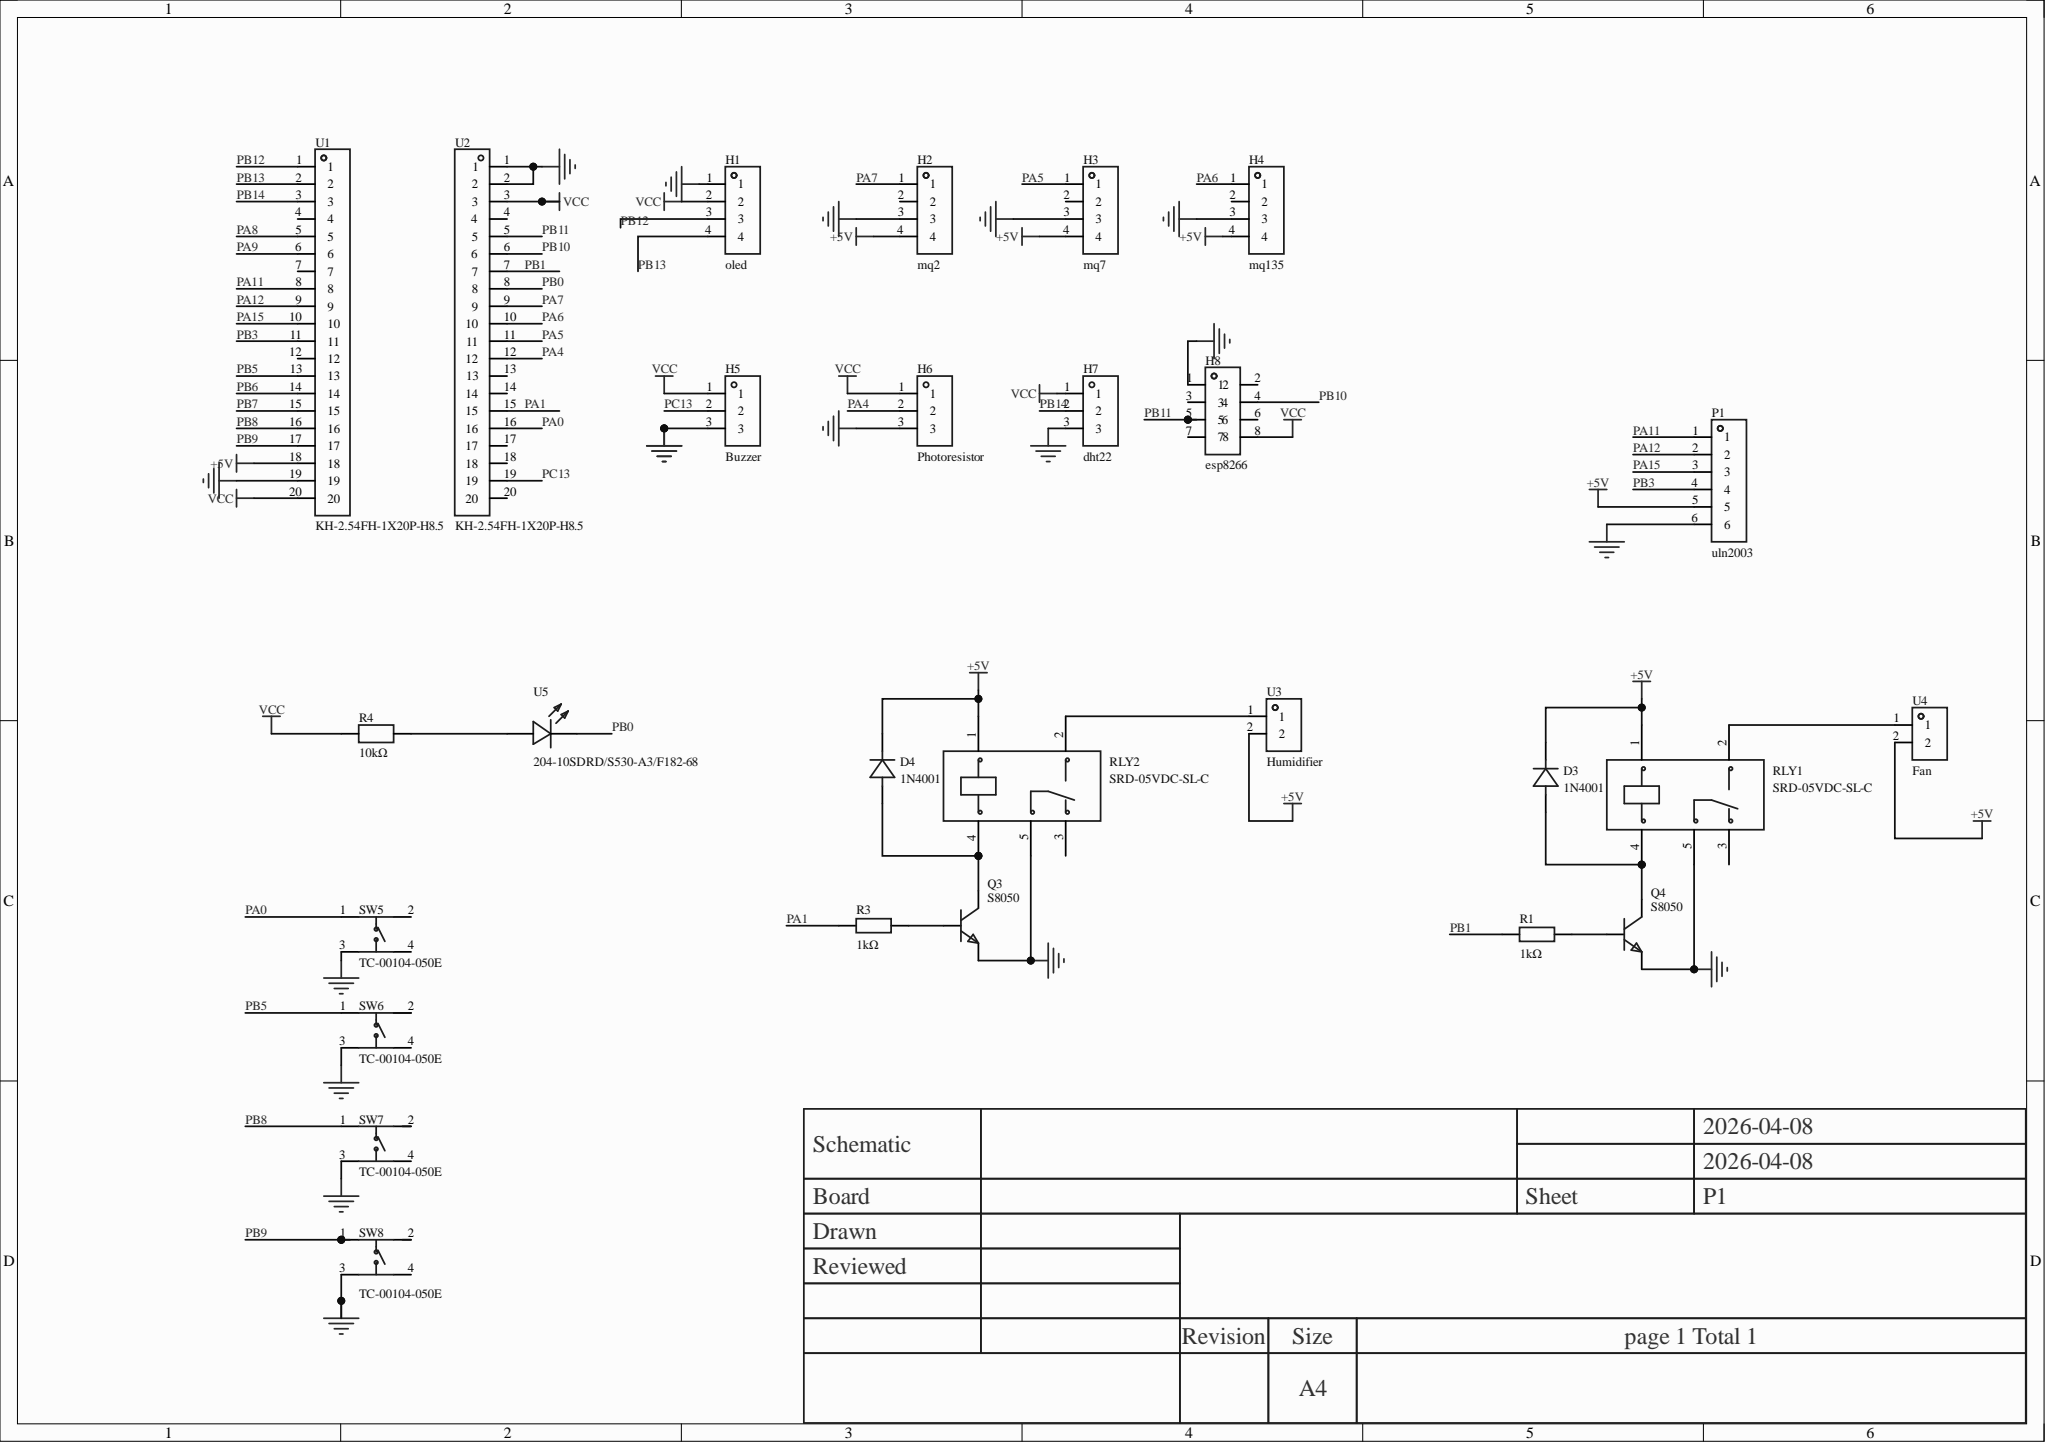Circuit board | Altium Designer | 27 parts | 31 nets
Bill of materials:
Comment,Description,Designator,Footprint,LibRef,Quantity
"1N4001","Diode configuration: independent; forward voltage drop (Vf): 1V@1A; DC reverse withstand voltage (Vr): 50V; rectified current: 1A;","D3, D4","DO-41_BD2.4-L4.7-P8.70-D0.9-RD","1N4001_C5359862","2"
"oled","Socket structure: 1x4P; pitch: 2.54mm; row spacing: -; round/square hole: square hole; mounting: through-hole; rows: single row; total positions: 4P; rated current: 3A; rated voltage: -; hole direction: top; plastic height: -; contact material: bronze; contact plating: -; operating temperature: -40℃~+105℃;","H1","HDR-TH_4P-P2.54-V-F","2.54-1*4P母","1"
"mq2","Socket structure: 1x4P; pitch: 2.54mm; row spacing: -; round/square hole: square hole; mounting: through-hole; rows: single row; total positions: 4P; rated current: 3A; rated voltage: -; hole direction: top; plastic height: -; contact material: bronze; contact plating: -; operating temperature: -40℃~+105℃;","H2","HDR-TH_4P-P2.54-V-F","2.54-1*4P母","1"
"mq7","Socket structure: 1x4P; pitch: 2.54mm; row spacing: -; round/square hole: square hole; mounting: through-hole; rows: single row; total positions: 4P; rated current: 3A; rated voltage: -; hole direction: top; plastic height: -; contact material: bronze; contact plating: -; operating temperature: -40℃~+105℃;","H3","HDR-TH_4P-P2.54-V-F","2.54-1*4P母","1"
"mq135","Socket structure: 1x4P; pitch: 2.54mm; row spacing: -; round/square hole: square hole; mounting: through-hole; rows: single row; total positions: 4P; rated current: 3A; rated voltage: -; hole direction: top; plastic height: -; contact material: bronze; contact plating: -; operating temperature: -40℃~+105℃;","H4","HDR-TH_4P-P2.54-V-F","2.54-1*4P母","1"
"Buzzer","Socket structure: 1x3P; pitch: 2.54mm; row spacing: -; round/square hole: square hole; mounting: through-hole; rows: single row; total positions: 3P; rated current: 3A; hole direction: top; plastic height: 8.5mm; contact material: brass; contact plating: -; operating temperature: -40℃~+105℃;","H5","HDR-TH_3P-P2.54-V-F","PM254V-11-03-H85","1"
"Photoresistor","Socket structure: 1x3P; pitch: 2.54mm; row spacing: -; round/square hole: square hole; mounting: through-hole; rows: single row; total positions: 3P; rated current: 3A; hole direction: top; plastic height: 8.5mm; contact material: brass; contact plating: -; operating temperature: -40℃~+105℃;","H6","HDR-TH_3P-P2.54-V-F","PM254V-11-03-H85","1"
"dht22","Socket structure: 1x3P; pitch: 2.54mm; row spacing: -; round/square hole: square hole; mounting: through-hole; rows: single row; total positions: 3P; rated current: 3A; hole direction: top; plastic height: 8.5mm; contact material: brass; contact plating: -; operating temperature: -40℃~+105℃;","H7","HDR-TH_3P-P2.54-V-F","PM254V-11-03-H85","1"
"esp8266","Socket structure: 2x4P; pitch: 2.54mm; row spacing: 2.54mm; round/square hole: square hole; mounting: through-hole; rows: double row; total positions: 8P; rated current: 3A; rated voltage: 250V; hole direction: top; plastic height: 8.5mm; operating temperature: -40℃~+105℃;","H8","HDR-TH_8P-P2.54-V-F-R2-C4-S2.54","PM254V-12-08-H85","1"
"uln2003","Socket structure: 1x6P; pitch: 2.54mm; row spacing: -; round/square hole: square hole; mounting: through-hole; rows: single row; total positions: 6P; rated current: 3A; rated voltage: -; hole direction: top; plastic height: -; contact material: brass; contact plating: -; operating temperature: -40℃~+105℃;","P1","HDR-TH_6P-P2.54-V-F","2.54-1*6P母","1"
"S8050","Transistor type: NPN; collector current (Ic): 500mA; collector-emitter breakdown voltage (Vceo): 25V; power dissipation (Pd): 625mW; DC current gain (hFE): 160@50mA,1V;","Q3, Q4","TO-92-3_L4.5-W3.5-P1.27-L","S8050_C2931492","2"
"1kΩ","Resistor type: metal film resistor; resistance: 1kΩ; tolerance: ±1%; power: 250mW; temperature coefficient: ±50ppm/?;","R1, R3","RES-TH_BD2.5-L6.5-P10.50-D0.6","MFR0W4F1001A50","2"
"10kΩ","Resistor type: metal film resistor; resistance: 10kΩ; tolerance: ±1%; power: 250mW; temperature coefficient: ±100ppm/?;","R4","RES-TH_BD2.7-L6.2-P10.20-D0.4","MF1/4W-10K±1%-ST52","1"
"SRD-05VDC-SL-C","Coil voltage: 5V; contact form: changeover 1C (SPDT); contact rating (resistive load): -; max switching voltage: 250V@AC; max switching current: 15A;","RLY1, RLY2","RELAY-TH_SRD-XXVDC-XL-C","SRD-05VDC-SL-C","2"
"TC-00104-050E","Circuit structure: SPST; button shape: round button; actuation force: 2.5N; mounting: through-hole; switch length: 6mm; switch width: 6mm; switch height: 5mm; bracket: without bracket; lamp: none; operating life: -;","SW5, SW6, SW7, SW8","SW-TH_4P-L6.0-W6.0-P4.50-LS6.5","TC-00104-050E","4"
"KH-2.54FH-1X20P-H8.5","Socket structure: 1x20P; pitch: 2.54mm; row spacing: -; round/square hole: square hole; mounting: through-hole; rows: single row; total positions: 20P; rated current: 3A; rated voltage: -; hole direction: top; plastic height: 8.5mm; operating temperature: -40℃~+105℃;","U1, U2","HDR-TH_20P-P2.54-V-F-2","KH-2.54FH-1X20P-H8.5","2"
"Humidifier","Socket structure: 1x2P; pitch: 2.54mm; row spacing: -; round/square hole: square hole; mounting: through-hole; rows: single row; total positions: 2P; rated current: 3A; rated voltage: -; hole direction: top; plastic height: 8.5mm; contact material: brass; contact plating: gold; operating temperature: -40℃~+105℃;","U3","HDR-TH_2P-P2.54-V-F","ZX-PM2.54-1-2PY","1"
"Fan","Socket structure: 1x2P; pitch: 2.54mm; row spacing: -; round/square hole: square hole; mounting: through-hole; rows: single row; total positions: 2P; rated current: 3A; rated voltage: -; hole direction: top; plastic height: 8.5mm; contact material: brass; contact plating: gold; operating temperature: -40℃~+105℃;","U4","HDR-TH_2P-P2.54-V-F","ZX-PM2.54-1-2PY","1"
"204-10SDRD/S530-A3/F182-68","-","U5","LED-TH_BD4.0-P2.50-RD","204-10SDRD/S530-A3/F182-68","1"
Netlist (Protel format):
[
D3
DO-41_BD2.4-L4.7-P8.70-D0.9-RD
1N4001



]
[
D4
DO-41_BD2.4-L4.7-P8.70-D0.9-RD
1N4001



]
[
H1
HDR-TH_4P-P2.54-V-F
oled



]
[
H2
HDR-TH_4P-P2.54-V-F
mq2



]
[
H3
HDR-TH_4P-P2.54-V-F
mq7



]
[
H4
HDR-TH_4P-P2.54-V-F
mq135



]
[
H5
HDR-TH_3P-P2.54-V-F
Buzzer



]
[
H6
HDR-TH_3P-P2.54-V-F
Photoresistor



]
[
H7
HDR-TH_3P-P2.54-V-F
dht22



]
[
H8
HDR-TH_8P-P2.54-V-F-R2-C4-S2.54
esp8266



]
[
P1
HDR-TH_6P-P2.54-V-F
uln2003



]
[
Q3
TO-92-3_L4.5-W3.5-P1.27-L
S8050



]
[
Q4
TO-92-3_L4.5-W3.5-P1.27-L
S8050



]
[
R1
RES-TH_BD2.5-L6.5-P10.50-D0.6
1kΩ



]
[
R3
RES-TH_BD2.5-L6.5-P10.50-D0.6
1kΩ



]
[
R4
RES-TH_BD2.7-L6.2-P10.20-D0.4
10kΩ



]
[
RLY1
RELAY-TH_SRD-XXVDC-XL-C
SRD-05VDC-SL-C



]
[
RLY2
RELAY-TH_SRD-XXVDC-XL-C
SRD-05VDC-SL-C



]
[
SW5
SW-TH_4P-L6.0-W6.0-P4.50-LS6.5
TC-00104-050E



]
[
SW6
SW-TH_4P-L6.0-W6.0-P4.50-LS6.5
TC-00104-050E



]
[
SW7
SW-TH_4P-L6.0-W6.0-P4.50-LS6.5
TC-00104-050E



]
[
SW8
SW-TH_4P-L6.0-W6.0-P4.50-LS6.5
TC-00104-050E



]
[
U1
HDR-TH_20P-P2.54-V-F-2
KH-2.54FH-1X20P-H8.5



]
[
U2
HDR-TH_20P-P2.54-V-F-2
KH-2.54FH-1X20P-H8.5



]
[
U3
HDR-TH_2P-P2.54-V-F
Humidifier



]
[
U4
HDR-TH_2P-P2.54-V-F
Fan



]
[
U5
LED-TH_BD4.0-P2.50-RD
204-10SDRD/S530-A3/F182-68



]
(
VCC
H1-2
H5-1
H6-1
H7-1
H8-8
R4-1
U1-20
U2-3
)
(
PC13
H5-2
U2-19
)
(
PB14
H7-2
U1-3
)
(
PB13
H1-4
U1-2
)
(
PB12
H1-3
U1-1
)
(
PB11
H8-5
U2-5
)
(
PB10
H8-4
U2-6
)
(
PB9
SW8-1
U1-17
)
(
PB8
SW7-1
U1-16
)
(
PB5
SW6-1
U1-13
)
(
PB3
P1-4
U1-11
)
(
PB1
R1-1
U2-7
)
(
PB0
U2-8
U5-1
)
(
PA15
P1-3
U1-10
)
(
PA12
P1-2
U1-9
)
(
PA11
P1-1
U1-8
)
(
PA7
H2-1
U2-9
)
(
PA6
H4-1
U2-10
)
(
PA5
H3-1
U2-11
)
(
PA4
H6-2
U2-12
)
(
PA1
R3-1
U2-15
)
(
PA0
SW5-1
U2-16
)
(
NetRLY2_2
RLY2-2
U3-1
)
(
NetRLY1_2
RLY1-2
U4-1
)
(
NetR4_2
R4-2
U5-2
)
(
NetQ4_2
Q4-2
R1-2
)
(
NetQ3_2
Q3-2
R3-2
)
(
NetD4_2
D4-2
Q3-3
RLY2-4
)
(
NetD3_2
D3-2
Q4-3
RLY1-4
)
(
GND
H1-1
H2-3
H3-3
H4-3
H5-3
H6-3
H7-3
H8-1
P1-6
Q3-1
Q4-1
RLY1-5
RLY2-5
SW5-3
SW6-3
SW7-3
SW8-3
U1-19
U2-1
U2-2
)
(
+5V
D3-1
D4-1
H2-4
H3-4
H4-4
P1-5
RLY1-1
RLY2-1
U1-18
U3-2
U4-2
)